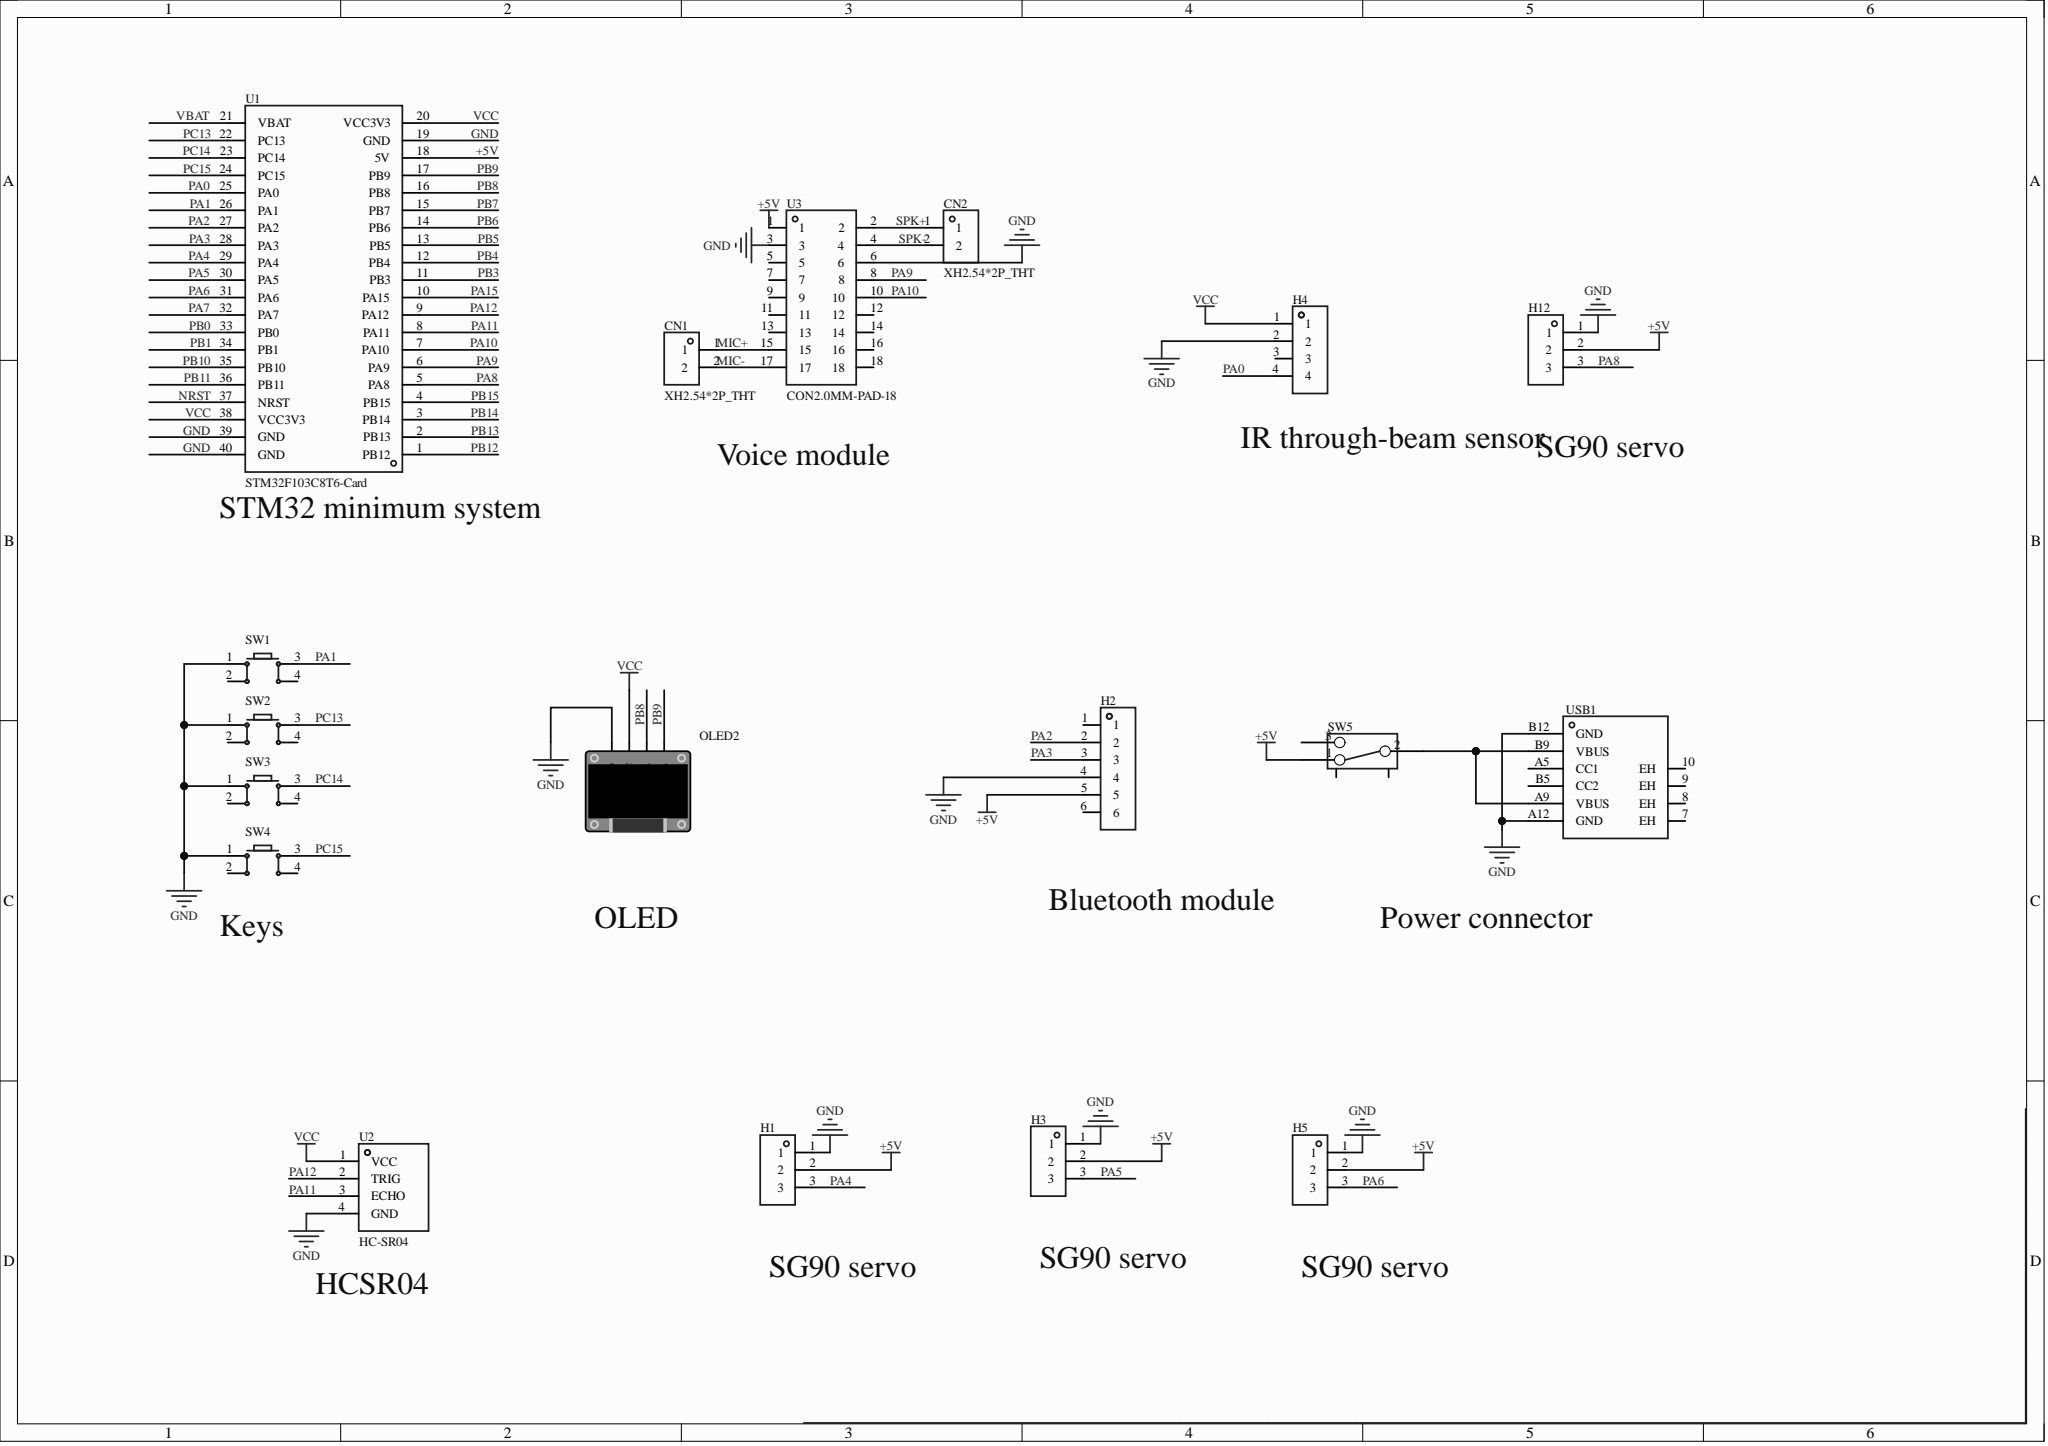Circuit board | Altium Designer | 18 parts | 25 nets
Bill of materials:
Comment,Description,Designator,Footprint,LibRef,Quantity
"XH2.54*2P_THT","","CN1, CN2","CONN-TH_2P-P2.50-XH2.54-2P","XH2.54*2P_直插","2"
"","","H1, H3, H5, H12","HDR-TH_3P-P2.54-V-F","HDR-F_2.54_1x3P","4"
"","","H2","HDR-TH_6P-P2.54-V-F","HDR-F_2.54_1x6P","1"
"","","H4","HDR-TH_4P-P2.54-V-F","HDR-F_2.54_1x4P","1"
"","","OLED2","0.96OLED_4P","0.96OLED模块_4P","1"
"","","SW1, SW2, SW3, SW4","SW-TH_4P-L6.0-W6.0-P4.50-LS6.5","Key_TH_6x6x6","4"
"","","SW5","拨动开关","拨动开关_正","1"
"STM32F103C8T6-Card","","U1","CONN-TH_L53.3-W22.9_STM32F103C8T6-CARD","STM32F103C8T6-Card","1"
"HC-SR04","","U2","TH_HC-SR04V","HC-SR04","1"
"CON2.0MM-PAD-18","","U3","CONN-TH_18P-P2.00_C9900078766","CON2.0MM-PAD-18","1"
"","","USB1","USB_ TYPE-C-6P","USB_ Type-C-6P","1"
Netlist (Protel format):
[
CN1
CONN-TH_2P-P2.50-XH2.54-2P
XH2.54*2P_THT



]
[
CN2
CONN-TH_2P-P2.50-XH2.54-2P
XH2.54*2P_THT



]
[
H1
HDR-TH_3P-P2.54-V-F




]
[
H2
HDR-TH_6P-P2.54-V-F




]
[
H3
HDR-TH_3P-P2.54-V-F




]
[
H4
HDR-TH_4P-P2.54-V-F




]
[
H5
HDR-TH_3P-P2.54-V-F




]
[
H12
HDR-TH_3P-P2.54-V-F




]
[
OLED2
0.96OLED_4P




]
[
SW1
SW-TH_4P-L6.0-W6.0-P4.50-LS6.5




]
[
SW2
SW-TH_4P-L6.0-W6.0-P4.50-LS6.5




]
[
SW3
SW-TH_4P-L6.0-W6.0-P4.50-LS6.5




]
[
SW4
SW-TH_4P-L6.0-W6.0-P4.50-LS6.5




]
[
SW5
拨动开关




]
[
U1
CONN-TH_L53.3-W22.9_STM32F103C8T6-CARD
STM32F103C8T6-Card



]
[
U2
TH_HC-SR04V
HC-SR04



]
[
U3
CONN-TH_18P-P2.00_C9900078766
CON2.0MM-PAD-18



]
[
USB1
USB_ TYPE-C-6P




]
(
VCC
H4-1
OLED2-2
U1-20
U1-38
U2-1
)
(
SPK-
CN2-2
U3-4
)
(
SPK+
CN2-1
U3-2
)
(
PC15
SW4-3
U1-24
)
(
PC14
SW3-3
U1-23
)
(
PC13
SW2-3
U1-22
)
(
PB9
OLED2-4
U1-17
)
(
PB8
OLED2-3
U1-16
)
(
PA12
U1-9
U2-2
)
(
PA11
U1-8
U2-3
)
(
PA10
U1-7
U3-10
)
(
PA9
U1-6
U3-8
)
(
PA8
H12-3
U1-5
)
(
PA6
H5-3
U1-31
)
(
PA5
H3-3
U1-30
)
(
PA4
H1-3
U1-29
)
(
PA3
H2-3
U1-28
)
(
PA2
H2-2
U1-27
)
(
PA1
SW1-3
U1-26
)
(
PA0
H4-4
U1-25
)
(
NetSW5_2
SW5-2
USB1-A9
USB1-B9
)
(
MIC-
CN1-2
U3-17
)
(
MIC+
CN1-1
U3-15
)
(
GND
H1-1
H2-4
H3-1
H4-2
H5-1
H12-1
OLED2-1
SW1-1
SW2-1
SW3-1
SW4-1
U1-19
U1-39
U1-40
U2-4
U3-3
U3-6
USB1-A12
USB1-B12
)
(
+5V
H1-2
H2-5
H3-2
H5-2
H12-2
SW5-1
U1-18
U3-1
)